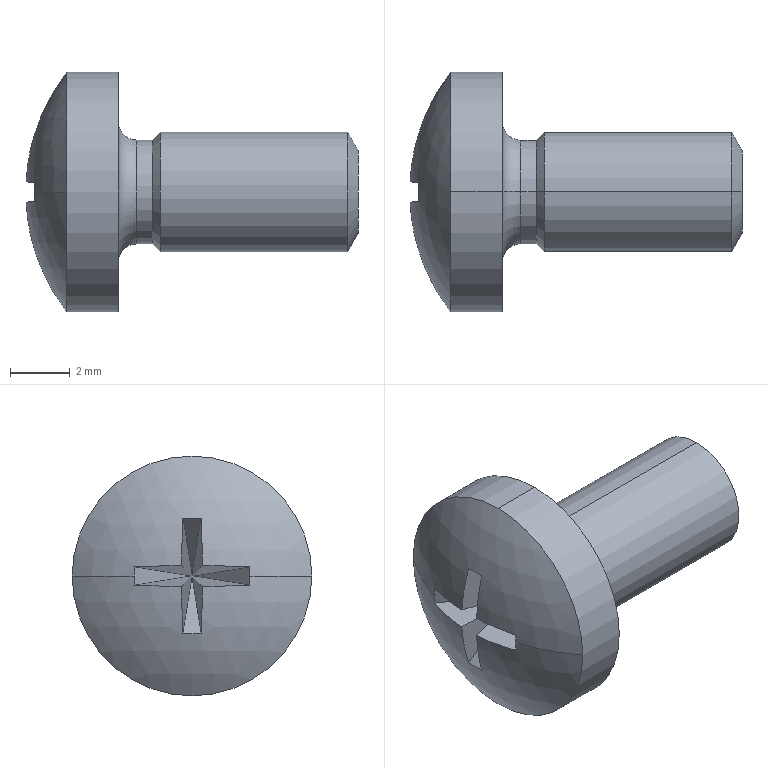Part | SolidWorks | features BlendCut 1, LPattern 1, MirrorPattern 1, RevCut 1, Revolution 1 | 1 solid | 28 faces | box 11.081 x 8 x 8 mm | volume 215 mm3 | plane 14 | cylinder 6 | cone 4 | torus 2 | sphere 2 | commonest cylinder face diameters 3.464 x2 4 x2 8 x2
STEP:
#1=CARTESIAN_POINT('',(11.1,0.,1.394));
#2=VERTEX_POINT('',#1);
#3=CARTESIAN_POINT('',(11.1,0.,-1.394));
#4=VERTEX_POINT('',#3);
#5=CARTESIAN_POINT('',(11.1,0.,0.));
#6=DIRECTION('',(-1.,0.,0.));
#7=DIRECTION('',(0.,0.,1.));
#8=AXIS2_PLACEMENT_3D('',#5,#6,#7);
#9=CIRCLE('',#8,1.394);
#10=EDGE_CURVE('',#2,#4,#9,.T.);
#11=ORIENTED_EDGE('',*,*,#10,.T.);
#12=CARTESIAN_POINT('',(10.754,0.,-2.));
#13=VERTEX_POINT('',#12);
#14=CARTESIAN_POINT('',(10.754,0.,-2.));
#15=DIRECTION('',(-0.4959,0.,-0.8684));
#16=VECTOR('',#15,1000.);
#17=LINE('',#14,#16);
#18=EDGE_CURVE('',#4,#13,#17,.T.);
#19=ORIENTED_EDGE('',*,*,#18,.T.);
#20=CARTESIAN_POINT('',(10.754,0.,2.));
#21=VERTEX_POINT('',#20);
#22=CARTESIAN_POINT('',(10.754,0.,0.));
#23=DIRECTION('',(-1.,0.,0.));
#24=DIRECTION('',(0.,0.,1.));
#25=AXIS2_PLACEMENT_3D('',#22,#23,#24);
#26=CIRCLE('',#25,2.);
#27=EDGE_CURVE('',#21,#13,#26,.T.);
#28=ORIENTED_EDGE('',*,*,#27,.F.);
#29=CARTESIAN_POINT('',(10.754,0.,2.));
#30=DIRECTION('',(-0.4959,0.,0.8684));
#31=VECTOR('',#30,1000.);
#32=LINE('',#29,#31);
#33=EDGE_CURVE('',#2,#21,#32,.T.);
#34=ORIENTED_EDGE('',*,*,#33,.F.);
#35=EDGE_LOOP('',(#11,#19,#28,#34));
#36=FACE_OUTER_BOUND('',#35,.T.);
#37=CARTESIAN_POINT('',(10.754,0.,0.));
#38=DIRECTION('',(-1.,0.,0.));
#39=DIRECTION('',(0.,0.,1.));
#40=AXIS2_PLACEMENT_3D('',#37,#38,#39);
#41=CONICAL_SURFACE('',#40,2.,1.052);
#42=ADVANCED_FACE('',(#36),#41,.T.);
#43=CARTESIAN_POINT('',(4.232,0.,1.732));
#44=VERTEX_POINT('',#43);
#45=CARTESIAN_POINT('',(4.232,0.,-1.732));
#46=VERTEX_POINT('',#45);
#47=CARTESIAN_POINT('',(4.232,0.,0.));
#48=DIRECTION('',(-1.,0.,0.));
#49=DIRECTION('',(0.,0.,1.));
#50=AXIS2_PLACEMENT_3D('',#47,#48,#49);
#51=CIRCLE('',#50,1.732);
#52=EDGE_CURVE('',#44,#46,#51,.T.);
#53=ORIENTED_EDGE('',*,*,#52,.F.);
#54=CARTESIAN_POINT('',(4.5,0.,2.));
#55=VERTEX_POINT('',#54);
#56=CARTESIAN_POINT('',(4.5,0.,2.));
#57=DIRECTION('',(0.7071,0.,0.7071));
#58=VECTOR('',#57,1000.);
#59=LINE('',#56,#58);
#60=EDGE_CURVE('',#44,#55,#59,.T.);
#61=ORIENTED_EDGE('',*,*,#60,.T.);
#62=CARTESIAN_POINT('',(4.5,0.,-2.));
#63=VERTEX_POINT('',#62);
#64=CARTESIAN_POINT('',(4.5,0.,0.));
#65=DIRECTION('',(-1.,0.,0.));
#66=DIRECTION('',(0.,0.,1.));
#67=AXIS2_PLACEMENT_3D('',#64,#65,#66);
#68=CIRCLE('',#67,2.);
#69=EDGE_CURVE('',#55,#63,#68,.T.);
#70=ORIENTED_EDGE('',*,*,#69,.T.);
#71=CARTESIAN_POINT('',(4.5,0.,-2.));
#72=DIRECTION('',(0.7071,0.,-0.7071));
#73=VECTOR('',#72,1000.);
#74=LINE('',#71,#73);
#75=EDGE_CURVE('',#46,#63,#74,.T.);
#76=ORIENTED_EDGE('',*,*,#75,.F.);
#77=EDGE_LOOP('',(#53,#61,#70,#76));
#78=FACE_OUTER_BOUND('',#77,.T.);
#79=CARTESIAN_POINT('',(4.5,0.,0.));
#80=DIRECTION('',(1.,0.,0.));
#81=DIRECTION('',(0.,0.,-1.));
#82=AXIS2_PLACEMENT_3D('',#79,#80,#81);
#83=CONICAL_SURFACE('',#82,2.,0.7854);
#84=ADVANCED_FACE('',(#78),#83,.T.);
#85=ORIENTED_EDGE('',*,*,#52,.T.);
#86=CARTESIAN_POINT('',(3.718,0.,-1.732));
#87=VERTEX_POINT('',#86);
#88=CARTESIAN_POINT('',(-1.332,0.,-1.732));
#89=DIRECTION('',(-1.,0.,0.));
#90=VECTOR('',#89,1000.);
#91=LINE('',#88,#90);
#92=EDGE_CURVE('',#46,#87,#91,.T.);
#93=ORIENTED_EDGE('',*,*,#92,.T.);
#94=CARTESIAN_POINT('',(3.718,0.,1.732));
#95=VERTEX_POINT('',#94);
#96=CARTESIAN_POINT('',(3.718,0.,0.));
#97=DIRECTION('',(-1.,0.,0.));
#98=DIRECTION('',(0.,0.,1.));
#99=AXIS2_PLACEMENT_3D('',#96,#97,#98);
#100=CIRCLE('',#99,1.732);
#101=EDGE_CURVE('',#95,#87,#100,.T.);
#102=ORIENTED_EDGE('',*,*,#101,.F.);
#103=CARTESIAN_POINT('',(-1.332,0.,1.732));
#104=DIRECTION('',(-1.,0.,0.));
#105=VECTOR('',#104,1000.);
#106=LINE('',#103,#105);
#107=EDGE_CURVE('',#44,#95,#106,.T.);
#108=ORIENTED_EDGE('',*,*,#107,.F.);
#109=EDGE_LOOP('',(#85,#93,#102,#108));
#110=FACE_OUTER_BOUND('',#109,.T.);
#111=CARTESIAN_POINT('',(-1.332,0.,0.));
#112=DIRECTION('',(-1.,0.,0.));
#113=DIRECTION('',(0.,0.,1.));
#114=AXIS2_PLACEMENT_3D('',#111,#112,#113);
#115=CYLINDRICAL_SURFACE('',#114,1.732);
#116=ADVANCED_FACE('',(#110),#115,.T.);
#117=CARTESIAN_POINT('',(3.1,0.,-2.35));
#118=VERTEX_POINT('',#117);
#119=CARTESIAN_POINT('',(3.1,0.,2.35));
#120=VERTEX_POINT('',#119);
#121=CARTESIAN_POINT('',(3.1,0.,0.));
#122=DIRECTION('',(-1.,0.,0.));
#123=DIRECTION('',(0.,0.,1.));
#124=AXIS2_PLACEMENT_3D('',#121,#122,#123);
#125=CIRCLE('',#124,2.35);
#126=EDGE_CURVE('',#118,#120,#125,.T.);
#127=ORIENTED_EDGE('',*,*,#126,.F.);
#128=CARTESIAN_POINT('',(3.718,0.,-2.35));
#129=DIRECTION('',(0.,1.,0.));
#130=DIRECTION('',(0.,0.,1.));
#131=AXIS2_PLACEMENT_3D('',#128,#129,#130);
#132=CIRCLE('',#131,0.618);
#133=EDGE_CURVE('',#118,#87,#132,.T.);
#134=ORIENTED_EDGE('',*,*,#133,.T.);
#135=CARTESIAN_POINT('',(3.718,0.,0.));
#136=DIRECTION('',(-1.,0.,0.));
#137=DIRECTION('',(0.,0.,1.));
#138=AXIS2_PLACEMENT_3D('',#135,#136,#137);
#139=CIRCLE('',#138,1.732);
#140=EDGE_CURVE('',#87,#95,#139,.T.);
#141=ORIENTED_EDGE('',*,*,#140,.T.);
#142=CARTESIAN_POINT('',(3.718,0.,2.35));
#143=DIRECTION('',(0.,-1.,0.));
#144=DIRECTION('',(0.,0.,-1.));
#145=AXIS2_PLACEMENT_3D('',#142,#143,#144);
#146=CIRCLE('',#145,0.618);
#147=EDGE_CURVE('',#120,#95,#146,.T.);
#148=ORIENTED_EDGE('',*,*,#147,.F.);
#149=EDGE_LOOP('',(#127,#134,#141,#148));
#150=FACE_OUTER_BOUND('',#149,.T.);
#151=CARTESIAN_POINT('',(3.718,0.,0.));
#152=DIRECTION('',(-1.,0.,0.));
#153=DIRECTION('',(0.,0.,1.));
#154=AXIS2_PLACEMENT_3D('',#151,#152,#153);
#155=TOROIDAL_SURFACE('',#154,2.35,0.618);
#156=ADVANCED_FACE('',(#150),#155,.F.);
#157=CARTESIAN_POINT('',(3.1,0.,4.));
#158=VERTEX_POINT('',#157);
#159=CARTESIAN_POINT('',(3.1,0.,-4.));
#160=VERTEX_POINT('',#159);
#161=CARTESIAN_POINT('',(3.1,0.,0.));
#162=DIRECTION('',(-1.,0.,0.));
#163=DIRECTION('',(0.,0.,1.));
#164=AXIS2_PLACEMENT_3D('',#161,#162,#163);
#165=CIRCLE('',#164,4.);
#166=EDGE_CURVE('',#158,#160,#165,.T.);
#167=ORIENTED_EDGE('',*,*,#166,.T.);
#168=CARTESIAN_POINT('',(1.377,0.,-4.));
#169=VERTEX_POINT('',#168);
#170=CARTESIAN_POINT('',(-1.332,0.,-4.));
#171=DIRECTION('',(-1.,0.,0.));
#172=VECTOR('',#171,1000.);
#173=LINE('',#170,#172);
#174=EDGE_CURVE('',#160,#169,#173,.T.);
#175=ORIENTED_EDGE('',*,*,#174,.T.);
#176=CARTESIAN_POINT('',(1.377,4.,0.));
#177=VERTEX_POINT('',#176);
#178=CARTESIAN_POINT('',(1.377,0.,0.));
#179=DIRECTION('',(-1.,0.,0.));
#180=DIRECTION('',(0.,0.,1.));
#181=AXIS2_PLACEMENT_3D('',#178,#179,#180);
#182=CIRCLE('',#181,4.);
#183=EDGE_CURVE('',#177,#169,#182,.T.);
#184=ORIENTED_EDGE('',*,*,#183,.F.);
#185=CARTESIAN_POINT('',(1.377,0.,4.));
#186=VERTEX_POINT('',#185);
#187=CARTESIAN_POINT('',(1.377,0.,0.));
#188=DIRECTION('',(-1.,0.,0.));
#189=DIRECTION('',(0.,0.,1.));
#190=AXIS2_PLACEMENT_3D('',#187,#188,#189);
#191=CIRCLE('',#190,4.);
#192=EDGE_CURVE('',#186,#177,#191,.T.);
#193=ORIENTED_EDGE('',*,*,#192,.F.);
#194=CARTESIAN_POINT('',(-1.332,0.,4.));
#195=DIRECTION('',(-1.,0.,0.));
#196=VECTOR('',#195,1000.);
#197=LINE('',#194,#196);
#198=EDGE_CURVE('',#158,#186,#197,.T.);
#199=ORIENTED_EDGE('',*,*,#198,.F.);
#200=EDGE_LOOP('',(#167,#175,#184,#193,#199));
#201=FACE_OUTER_BOUND('',#200,.T.);
#202=CARTESIAN_POINT('',(-1.332,0.,0.));
#203=DIRECTION('',(-1.,0.,0.));
#204=DIRECTION('',(0.,0.,1.));
#205=AXIS2_PLACEMENT_3D('',#202,#203,#204);
#206=CYLINDRICAL_SURFACE('',#205,4.);
#207=ADVANCED_FACE('',(#201),#206,.T.);
#208=ORIENTED_EDGE('',*,*,#183,.T.);
#209=CARTESIAN_POINT('',(1.377,-4.,0.));
#210=VERTEX_POINT('',#209);
#211=CARTESIAN_POINT('',(1.377,0.,0.));
#212=DIRECTION('',(-1.,0.,0.));
#213=DIRECTION('',(0.,0.,1.));
#214=AXIS2_PLACEMENT_3D('',#211,#212,#213);
#215=CIRCLE('',#214,4.);
#216=EDGE_CURVE('',#169,#210,#215,.T.);
#217=ORIENTED_EDGE('',*,*,#216,.T.);
#218=CARTESIAN_POINT('',(0.2935,-1.931,0.));
#219=VERTEX_POINT('',#218);
#220=CARTESIAN_POINT('',(6.5,0.,0.));
#221=DIRECTION('',(0.,0.,-1.));
#222=DIRECTION('',(0.,1.,0.));
#223=AXIS2_PLACEMENT_3D('',#220,#221,#222);
#224=CIRCLE('',#223,6.5);
#225=EDGE_CURVE('',#210,#219,#224,.T.);
#226=ORIENTED_EDGE('',*,*,#225,.T.);
#227=CARTESIAN_POINT('',(0.2993,-1.926,-0.3063));
#228=VERTEX_POINT('',#227);
#229=CARTESIAN_POINT('',(4.628,2.042,0.));
#230=DIRECTION('',(0.6757,-0.7372,0.));
#231=DIRECTION('',(0.7372,0.6757,0.));
#232=AXIS2_PLACEMENT_3D('',#229,#230,#231);
#233=CIRCLE('',#232,5.88);
#234=EDGE_CURVE('',#219,#228,#233,.T.);
#235=ORIENTED_EDGE('',*,*,#234,.T.);
#236=CARTESIAN_POINT('',(0.01858,-0.3473,-0.3473));
#237=VERTEX_POINT('',#236);
#238=CARTESIAN_POINT('',(6.415,0.,0.5855));
#239=DIRECTION('',(0.1443,0.,-0.9895));
#240=DIRECTION('',(-0.9895,0.,-0.1443));
#241=AXIS2_PLACEMENT_3D('',#238,#239,#240);
#242=CIRCLE('',#241,6.473);
#243=EDGE_CURVE('',#228,#237,#242,.T.);
#244=ORIENTED_EDGE('',*,*,#243,.T.);
#245=CARTESIAN_POINT('',(0.2993,-0.3063,-1.926));
#246=VERTEX_POINT('',#245);
#247=CARTESIAN_POINT('',(6.415,0.5855,0.));
#248=DIRECTION('',(0.1443,-0.9895,0.));
#249=DIRECTION('',(0.9895,0.1443,0.));
#250=AXIS2_PLACEMENT_3D('',#247,#248,#249);
#251=CIRCLE('',#250,6.473);
#252=EDGE_CURVE('',#237,#246,#251,.T.);
#253=ORIENTED_EDGE('',*,*,#252,.T.);
#254=CARTESIAN_POINT('',(0.2993,0.3063,-1.926));
#255=VERTEX_POINT('',#254);
#256=CARTESIAN_POINT('',(4.628,0.,2.042));
#257=DIRECTION('',(0.6757,0.,-0.7372));
#258=DIRECTION('',(-0.7372,0.,-0.6757));
#259=AXIS2_PLACEMENT_3D('',#256,#257,#258);
#260=CIRCLE('',#259,5.88);
#261=EDGE_CURVE('',#246,#255,#260,.T.);
#262=ORIENTED_EDGE('',*,*,#261,.T.);
#263=CARTESIAN_POINT('',(0.01858,0.3473,-0.3473));
#264=VERTEX_POINT('',#263);
#265=CARTESIAN_POINT('',(6.415,-0.5855,0.));
#266=DIRECTION('',(0.1443,0.9895,0.));
#267=DIRECTION('',(-0.9895,0.1443,0.));
#268=AXIS2_PLACEMENT_3D('',#265,#266,#267);
#269=CIRCLE('',#268,6.473);
#270=EDGE_CURVE('',#255,#264,#269,.T.);
#271=ORIENTED_EDGE('',*,*,#270,.T.);
#272=CARTESIAN_POINT('',(0.2993,1.926,-0.3063));
#273=VERTEX_POINT('',#272);
#274=CARTESIAN_POINT('',(6.415,0.,0.5855));
#275=DIRECTION('',(0.1443,0.,-0.9895));
#276=DIRECTION('',(-0.9895,0.,-0.1443));
#277=AXIS2_PLACEMENT_3D('',#274,#275,#276);
#278=CIRCLE('',#277,6.473);
#279=EDGE_CURVE('',#264,#273,#278,.T.);
#280=ORIENTED_EDGE('',*,*,#279,.T.);
#281=CARTESIAN_POINT('',(0.2935,1.931,0.));
#282=VERTEX_POINT('',#281);
#283=CARTESIAN_POINT('',(4.628,-2.042,0.));
#284=DIRECTION('',(0.6757,0.7372,0.));
#285=DIRECTION('',(-0.7372,0.6757,0.));
#286=AXIS2_PLACEMENT_3D('',#283,#284,#285);
#287=CIRCLE('',#286,5.88);
#288=EDGE_CURVE('',#273,#282,#287,.T.);
#289=ORIENTED_EDGE('',*,*,#288,.T.);
#290=CARTESIAN_POINT('',(6.5,0.,0.));
#291=DIRECTION('',(0.,0.,1.));
#292=DIRECTION('',(1.,0.,0.));
#293=AXIS2_PLACEMENT_3D('',#290,#291,#292);
#294=CIRCLE('',#293,6.5);
#295=EDGE_CURVE('',#177,#282,#294,.T.);
#296=ORIENTED_EDGE('',*,*,#295,.F.);
#297=EDGE_LOOP('',(#208,#217,#226,#235,#244,#253,#262,#271,#280,#289,#296));
#298=FACE_OUTER_BOUND('',#297,.T.);
#299=CARTESIAN_POINT('',(6.5,0.,0.));
#300=DIRECTION('',(0.,0.,-1.));
#301=DIRECTION('',(0.,1.,0.));
#302=AXIS2_PLACEMENT_3D('',#299,#300,#301);
#303=SPHERICAL_SURFACE('',#302,6.5);
#304=ADVANCED_FACE('',(#298),#303,.T.);
#305=ORIENTED_EDGE('',*,*,#27,.T.);
#306=CARTESIAN_POINT('',(-1.332,0.,-2.));
#307=DIRECTION('',(-1.,0.,0.));
#308=VECTOR('',#307,1000.);
#309=LINE('',#306,#308);
#310=EDGE_CURVE('',#13,#63,#309,.T.);
#311=ORIENTED_EDGE('',*,*,#310,.T.);
#312=ORIENTED_EDGE('',*,*,#69,.F.);
#313=CARTESIAN_POINT('',(-1.332,0.,2.));
#314=DIRECTION('',(-1.,0.,0.));
#315=VECTOR('',#314,1000.);
#316=LINE('',#313,#315);
#317=EDGE_CURVE('',#21,#55,#316,.T.);
#318=ORIENTED_EDGE('',*,*,#317,.F.);
#319=EDGE_LOOP('',(#305,#311,#312,#318));
#320=FACE_OUTER_BOUND('',#319,.T.);
#321=CARTESIAN_POINT('',(-1.332,0.,0.));
#322=DIRECTION('',(-1.,0.,0.));
#323=DIRECTION('',(0.,0.,1.));
#324=AXIS2_PLACEMENT_3D('',#321,#322,#323);
#325=CYLINDRICAL_SURFACE('',#324,2.);
#326=ADVANCED_FACE('',(#320),#325,.T.);
#327=CARTESIAN_POINT('',(2.4,0.,0.));
#328=VERTEX_POINT('',#327);
#329=CARTESIAN_POINT('',(2.4,0.,0.));
#330=DIRECTION('',(-0.7329,-0.6719,-0.1069));
#331=VECTOR('',#330,1000.);
#332=LINE('',#329,#331);
#333=EDGE_CURVE('',#328,#228,#332,.T.);
#334=ORIENTED_EDGE('',*,*,#333,.F.);
#335=CARTESIAN_POINT('',(2.4,0.,0.));
#336=DIRECTION('',(-0.9794,-0.1428,-0.1428));
#337=VECTOR('',#336,1000.);
#338=LINE('',#335,#337);
#339=EDGE_CURVE('',#328,#237,#338,.T.);
#340=ORIENTED_EDGE('',*,*,#339,.T.);
#341=ORIENTED_EDGE('',*,*,#243,.F.);
#342=EDGE_LOOP('',(#334,#340,#341));
#343=FACE_OUTER_BOUND('',#342,.T.);
#344=CARTESIAN_POINT('',(2.4,0.,0.));
#345=DIRECTION('',(0.1443,0.,-0.9895));
#346=DIRECTION('',(-0.9895,0.,-0.1443));
#347=AXIS2_PLACEMENT_3D('',#344,#345,#346);
#348=PLANE('',#347);
#349=ADVANCED_FACE('',(#343),#348,.F.);
#350=CARTESIAN_POINT('',(0.01858,-0.3473,0.3473));
#351=VERTEX_POINT('',#350);
#352=CARTESIAN_POINT('',(0.2993,-1.926,0.3063));
#353=VERTEX_POINT('',#352);
#354=CARTESIAN_POINT('',(6.415,0.,-0.5855));
#355=DIRECTION('',(0.1443,0.,0.9895));
#356=DIRECTION('',(0.9895,0.,-0.1443));
#357=AXIS2_PLACEMENT_3D('',#354,#355,#356);
#358=CIRCLE('',#357,6.473);
#359=EDGE_CURVE('',#351,#353,#358,.T.);
#360=ORIENTED_EDGE('',*,*,#359,.F.);
#361=CARTESIAN_POINT('',(2.4,0.,0.));
#362=DIRECTION('',(0.9794,0.1428,-0.1428));
#363=VECTOR('',#362,1000.);
#364=LINE('',#361,#363);
#365=EDGE_CURVE('',#351,#328,#364,.T.);
#366=ORIENTED_EDGE('',*,*,#365,.T.);
#367=CARTESIAN_POINT('',(2.4,0.,0.));
#368=DIRECTION('',(-0.7329,-0.6719,0.1069));
#369=VECTOR('',#368,1000.);
#370=LINE('',#367,#369);
#371=EDGE_CURVE('',#328,#353,#370,.T.);
#372=ORIENTED_EDGE('',*,*,#371,.T.);
#373=EDGE_LOOP('',(#360,#366,#372));
#374=FACE_OUTER_BOUND('',#373,.T.);
#375=CARTESIAN_POINT('',(2.4,0.,0.));
#376=DIRECTION('',(0.1443,0.,0.9895));
#377=DIRECTION('',(0.9895,0.,-0.1443));
#378=AXIS2_PLACEMENT_3D('',#375,#376,#377);
#379=PLANE('',#378);
#380=ADVANCED_FACE('',(#374),#379,.F.);
#381=ORIENTED_EDGE('',*,*,#310,.F.);
#382=CARTESIAN_POINT('',(10.754,0.,0.));
#383=DIRECTION('',(-1.,0.,0.));
#384=DIRECTION('',(0.,0.,1.));
#385=AXIS2_PLACEMENT_3D('',#382,#383,#384);
#386=CIRCLE('',#385,2.);
#387=EDGE_CURVE('',#13,#21,#386,.T.);
#388=ORIENTED_EDGE('',*,*,#387,.T.);
#389=ORIENTED_EDGE('',*,*,#317,.T.);
#390=CARTESIAN_POINT('',(4.5,0.,0.));
#391=DIRECTION('',(-1.,0.,0.));
#392=DIRECTION('',(0.,0.,1.));
#393=AXIS2_PLACEMENT_3D('',#390,#391,#392);
#394=CIRCLE('',#393,2.);
#395=EDGE_CURVE('',#63,#55,#394,.T.);
#396=ORIENTED_EDGE('',*,*,#395,.F.);
#397=EDGE_LOOP('',(#381,#388,#389,#396));
#398=FACE_OUTER_BOUND('',#397,.T.);
#399=CARTESIAN_POINT('',(-1.332,0.,0.));
#400=DIRECTION('',(-1.,0.,0.));
#401=DIRECTION('',(0.,0.,1.));
#402=AXIS2_PLACEMENT_3D('',#399,#400,#401);
#403=CYLINDRICAL_SURFACE('',#402,2.);
#404=ADVANCED_FACE('',(#398),#403,.T.);
#405=ORIENTED_EDGE('',*,*,#225,.F.);
#406=CARTESIAN_POINT('',(1.377,0.,0.));
#407=DIRECTION('',(-1.,0.,0.));
#408=DIRECTION('',(0.,0.,1.));
#409=AXIS2_PLACEMENT_3D('',#406,#407,#408);
#410=CIRCLE('',#409,4.);
#411=EDGE_CURVE('',#210,#186,#410,.T.);
#412=ORIENTED_EDGE('',*,*,#411,.T.);
#413=ORIENTED_EDGE('',*,*,#192,.T.);
#414=ORIENTED_EDGE('',*,*,#295,.T.);
#415=CARTESIAN_POINT('',(0.2993,1.926,0.3063));
#416=VERTEX_POINT('',#415);
#417=CARTESIAN_POINT('',(4.628,-2.042,0.));
#418=DIRECTION('',(0.6757,0.7372,0.));
#419=DIRECTION('',(-0.7372,0.6757,0.));
#420=AXIS2_PLACEMENT_3D('',#417,#418,#419);
#421=CIRCLE('',#420,5.88);
#422=EDGE_CURVE('',#282,#416,#421,.T.);
#423=ORIENTED_EDGE('',*,*,#422,.T.);
#424=CARTESIAN_POINT('',(0.01858,0.3473,0.3473));
#425=VERTEX_POINT('',#424);
#426=CARTESIAN_POINT('',(6.415,0.,-0.5855));
#427=DIRECTION('',(0.1443,0.,0.9895));
#428=DIRECTION('',(0.9895,0.,-0.1443));
#429=AXIS2_PLACEMENT_3D('',#426,#427,#428);
#430=CIRCLE('',#429,6.473);
#431=EDGE_CURVE('',#416,#425,#430,.T.);
#432=ORIENTED_EDGE('',*,*,#431,.T.);
#433=CARTESIAN_POINT('',(0.2993,0.3063,1.926));
#434=VERTEX_POINT('',#433);
#435=CARTESIAN_POINT('',(6.415,-0.5855,0.));
#436=DIRECTION('',(0.1443,0.9895,0.));
#437=DIRECTION('',(-0.9895,0.1443,0.));
#438=AXIS2_PLACEMENT_3D('',#435,#436,#437);
#439=CIRCLE('',#438,6.473);
#440=EDGE_CURVE('',#425,#434,#439,.T.);
#441=ORIENTED_EDGE('',*,*,#440,.T.);
#442=CARTESIAN_POINT('',(0.2993,-0.3063,1.926));
#443=VERTEX_POINT('',#442);
#444=CARTESIAN_POINT('',(4.628,0.,-2.042));
#445=DIRECTION('',(0.6757,0.,0.7372));
#446=DIRECTION('',(0.7372,0.,-0.6757));
#447=AXIS2_PLACEMENT_3D('',#444,#445,#446);
#448=CIRCLE('',#447,5.88);
#449=EDGE_CURVE('',#434,#443,#448,.T.);
#450=ORIENTED_EDGE('',*,*,#449,.T.);
#451=CARTESIAN_POINT('',(6.415,0.5855,0.));
#452=DIRECTION('',(0.1443,-0.9895,0.));
#453=DIRECTION('',(0.9895,0.1443,0.));
#454=AXIS2_PLACEMENT_3D('',#451,#452,#453);
#455=CIRCLE('',#454,6.473);
#456=EDGE_CURVE('',#443,#351,#455,.T.);
#457=ORIENTED_EDGE('',*,*,#456,.T.);
#458=ORIENTED_EDGE('',*,*,#359,.T.);
#459=CARTESIAN_POINT('',(4.628,2.042,0.));
#460=DIRECTION('',(0.6757,-0.7372,0.));
#461=DIRECTION('',(0.7372,0.6757,0.));
#462=AXIS2_PLACEMENT_3D('',#459,#460,#461);
#463=CIRCLE('',#462,5.88);
#464=EDGE_CURVE('',#353,#219,#463,.T.);
#465=ORIENTED_EDGE('',*,*,#464,.T.);
#466=EDGE_LOOP('',(#405,#412,#413,#414,#423,#432,#441,#450,#457,#458,#465));
#467=FACE_OUTER_BOUND('',#466,.T.);
#468=CARTESIAN_POINT('',(6.5,0.,0.));
#469=DIRECTION('',(0.,0.,-1.));
#470=DIRECTION('',(0.,1.,0.));
#471=AXIS2_PLACEMENT_3D('',#468,#469,#470);
#472=SPHERICAL_SURFACE('',#471,6.5);
#473=ADVANCED_FACE('',(#467),#472,.T.);
#474=ORIENTED_EDGE('',*,*,#174,.F.);
#475=CARTESIAN_POINT('',(3.1,0.,0.));
#476=DIRECTION('',(-1.,0.,0.));
#477=DIRECTION('',(0.,0.,1.));
#478=AXIS2_PLACEMENT_3D('',#475,#476,#477);
#479=CIRCLE('',#478,4.);
#480=EDGE_CURVE('',#160,#158,#479,.T.);
#481=ORIENTED_EDGE('',*,*,#480,.T.);
#482=ORIENTED_EDGE('',*,*,#198,.T.);
#483=ORIENTED_EDGE('',*,*,#411,.F.);
#484=ORIENTED_EDGE('',*,*,#216,.F.);
#485=EDGE_LOOP('',(#474,#481,#482,#483,#484));
#486=FACE_OUTER_BOUND('',#485,.T.);
#487=CARTESIAN_POINT('',(-1.332,0.,0.));
#488=DIRECTION('',(-1.,0.,0.));
#489=DIRECTION('',(0.,0.,1.));
#490=AXIS2_PLACEMENT_3D('',#487,#488,#489);
#491=CYLINDRICAL_SURFACE('',#490,4.);
#492=ADVANCED_FACE('',(#486),#491,.T.);
#493=ORIENTED_EDGE('',*,*,#166,.F.);
#494=ORIENTED_EDGE('',*,*,#480,.F.);
#495=EDGE_LOOP('',(#493,#494));
#496=FACE_OUTER_BOUND('',#495,.T.);
#497=CARTESIAN_POINT('',(3.1,0.,0.));
#498=DIRECTION('',(-1.,0.,0.));
#499=DIRECTION('',(0.,0.,1.));
#500=AXIS2_PLACEMENT_3D('',#497,#498,#499);
#501=CIRCLE('',#500,2.35);
#502=EDGE_CURVE('',#120,#118,#501,.T.);
#503=ORIENTED_EDGE('',*,*,#502,.T.);
#504=ORIENTED_EDGE('',*,*,#126,.T.);
#505=EDGE_LOOP('',(#503,#504));
#506=FACE_BOUND('',#505,.T.);
#507=CARTESIAN_POINT('',(3.1,2.35,0.));
#508=DIRECTION('',(-1.,0.,0.));
#509=DIRECTION('',(0.,0.,1.));
#510=AXIS2_PLACEMENT_3D('',#507,#508,#509);
#511=PLANE('',#510);
#512=ADVANCED_FACE('',(#496,#506),#511,.F.);
#513=ORIENTED_EDGE('',*,*,#133,.F.);
#514=ORIENTED_EDGE('',*,*,#502,.F.);
#515=ORIENTED_EDGE('',*,*,#147,.T.);
#516=ORIENTED_EDGE('',*,*,#101,.T.);
#517=EDGE_LOOP('',(#513,#514,#515,#516));
#518=FACE_OUTER_BOUND('',#517,.T.);
#519=CARTESIAN_POINT('',(3.718,0.,0.));
#520=DIRECTION('',(-1.,0.,0.));
#521=DIRECTION('',(0.,0.,1.));
#522=AXIS2_PLACEMENT_3D('',#519,#520,#521);
#523=TOROIDAL_SURFACE('',#522,2.35,0.618);
#524=ADVANCED_FACE('',(#518),#523,.F.);
#525=ORIENTED_EDGE('',*,*,#92,.F.);
#526=CARTESIAN_POINT('',(4.232,0.,0.));
#527=DIRECTION('',(-1.,0.,0.));
#528=DIRECTION('',(0.,0.,1.));
#529=AXIS2_PLACEMENT_3D('',#526,#527,#528);
#530=CIRCLE('',#529,1.732);
#531=EDGE_CURVE('',#46,#44,#530,.T.);
#532=ORIENTED_EDGE('',*,*,#531,.T.);
#533=ORIENTED_EDGE('',*,*,#107,.T.);
#534=ORIENTED_EDGE('',*,*,#140,.F.);
#535=EDGE_LOOP('',(#525,#532,#533,#534));
#536=FACE_OUTER_BOUND('',#535,.T.);
#537=CARTESIAN_POINT('',(-1.332,0.,0.));
#538=DIRECTION('',(-1.,0.,0.));
#539=DIRECTION('',(0.,0.,1.));
#540=AXIS2_PLACEMENT_3D('',#537,#538,#539);
#541=CYLINDRICAL_SURFACE('',#540,1.732);
#542=ADVANCED_FACE('',(#536),#541,.T.);
#543=ORIENTED_EDGE('',*,*,#60,.F.);
#544=ORIENTED_EDGE('',*,*,#531,.F.);
#545=ORIENTED_EDGE('',*,*,#75,.T.);
#546=ORIENTED_EDGE('',*,*,#395,.T.);
#547=EDGE_LOOP('',(#543,#544,#545,#546));
#548=FACE_OUTER_BOUND('',#547,.T.);
#549=CARTESIAN_POINT('',(4.5,0.,0.));
#550=DIRECTION('',(1.,0.,0.));
#551=DIRECTION('',(0.,0.,-1.));
#552=AXIS2_PLACEMENT_3D('',#549,#550,#551);
#553=CONICAL_SURFACE('',#552,2.,0.7854);
#554=ADVANCED_FACE('',(#548),#553,.T.);
#555=ORIENTED_EDGE('',*,*,#18,.F.);
#556=CARTESIAN_POINT('',(11.1,0.,0.));
#557=DIRECTION('',(-1.,0.,0.));
#558=DIRECTION('',(0.,0.,1.));
#559=AXIS2_PLACEMENT_3D('',#556,#557,#558);
#560=CIRCLE('',#559,1.394);
#561=EDGE_CURVE('',#4,#2,#560,.T.);
#562=ORIENTED_EDGE('',*,*,#561,.T.);
#563=ORIENTED_EDGE('',*,*,#33,.T.);
#564=ORIENTED_EDGE('',*,*,#387,.F.);
#565=EDGE_LOOP('',(#555,#562,#563,#564));
#566=FACE_OUTER_BOUND('',#565,.T.);
#567=CARTESIAN_POINT('',(10.754,0.,0.));
#568=DIRECTION('',(-1.,0.,0.));
#569=DIRECTION('',(0.,0.,1.));
#570=AXIS2_PLACEMENT_3D('',#567,#568,#569);
#571=CONICAL_SURFACE('',#570,2.,1.052);
#572=ADVANCED_FACE('',(#566),#571,.T.);
#573=ORIENTED_EDGE('',*,*,#10,.F.);
#574=ORIENTED_EDGE('',*,*,#561,.F.);
#575=EDGE_LOOP('',(#573,#574));
#576=FACE_OUTER_BOUND('',#575,.T.);
#577=CARTESIAN_POINT('',(11.1,0.,0.));
#578=DIRECTION('',(-1.,0.,0.));
#579=DIRECTION('',(0.,0.,1.));
#580=AXIS2_PLACEMENT_3D('',#577,#578,#579);
#581=PLANE('',#580);
#582=ADVANCED_FACE('',(#576),#581,.F.);
#583=ORIENTED_EDGE('',*,*,#279,.F.);
#584=CARTESIAN_POINT('',(2.4,0.,0.));
#585=DIRECTION('',(0.9794,-0.1428,0.1428));
#586=VECTOR('',#585,1000.);
#587=LINE('',#584,#586);
#588=EDGE_CURVE('',#264,#328,#587,.T.);
#589=ORIENTED_EDGE('',*,*,#588,.T.);
#590=CARTESIAN_POINT('',(2.4,0.,0.));
#591=DIRECTION('',(-0.7329,0.6719,-0.1069));
#592=VECTOR('',#591,1000.);
#593=LINE('',#590,#592);
#594=EDGE_CURVE('',#328,#273,#593,.T.);
#595=ORIENTED_EDGE('',*,*,#594,.T.);
#596=EDGE_LOOP('',(#583,#589,#595));
#597=FACE_OUTER_BOUND('',#596,.T.);
#598=CARTESIAN_POINT('',(2.4,0.,0.));
#599=DIRECTION('',(0.1443,0.,-0.9895));
#600=DIRECTION('',(-0.9895,0.,-0.1443));
#601=AXIS2_PLACEMENT_3D('',#598,#599,#600);
#602=PLANE('',#601);
#603=ADVANCED_FACE('',(#597),#602,.F.);
#604=ORIENTED_EDGE('',*,*,#594,.F.);
#605=CARTESIAN_POINT('',(2.4,0.,0.));
#606=DIRECTION('',(-0.7329,0.6719,0.1069));
#607=VECTOR('',#606,1000.);
#608=LINE('',#605,#607);
#609=EDGE_CURVE('',#328,#416,#608,.T.);
#610=ORIENTED_EDGE('',*,*,#609,.T.);
#611=ORIENTED_EDGE('',*,*,#422,.F.);
#612=ORIENTED_EDGE('',*,*,#288,.F.);
#613=EDGE_LOOP('',(#604,#610,#611,#612));
#614=FACE_OUTER_BOUND('',#613,.T.);
#615=CARTESIAN_POINT('',(0.,2.2,-0.35));
#616=DIRECTION('',(0.6757,0.7372,0.));
#617=DIRECTION('',(-0.7372,0.6757,0.));
#618=AXIS2_PLACEMENT_3D('',#615,#616,#617);
#619=PLANE('',#618);
#620=ADVANCED_FACE('',(#614),#619,.F.);
#621=ORIENTED_EDGE('',*,*,#371,.F.);
#622=ORIENTED_EDGE('',*,*,#333,.T.);
#623=ORIENTED_EDGE('',*,*,#234,.F.);
#624=ORIENTED_EDGE('',*,*,#464,.F.);
#625=EDGE_LOOP('',(#621,#622,#623,#624));
#626=FACE_OUTER_BOUND('',#625,.T.);
#627=CARTESIAN_POINT('',(0.,-2.2,0.35));
#628=DIRECTION('',(0.6757,-0.7372,0.));
#629=DIRECTION('',(0.7372,0.6757,0.));
#630=AXIS2_PLACEMENT_3D('',#627,#628,#629);
#631=PLANE('',#630);
#632=ADVANCED_FACE('',(#626),#631,.F.);
#633=ORIENTED_EDGE('',*,*,#609,.F.);
#634=CARTESIAN_POINT('',(2.4,0.,0.));
#635=DIRECTION('',(-0.9794,0.1428,0.1428));
#636=VECTOR('',#635,1000.);
#637=LINE('',#634,#636);
#638=EDGE_CURVE('',#328,#425,#637,.T.);
#639=ORIENTED_EDGE('',*,*,#638,.T.);
#640=ORIENTED_EDGE('',*,*,#431,.F.);
#641=EDGE_LOOP('',(#633,#639,#640));
#642=FACE_OUTER_BOUND('',#641,.T.);
#643=CARTESIAN_POINT('',(2.4,0.,0.));
#644=DIRECTION('',(0.1443,0.,0.9895));
#645=DIRECTION('',(0.9895,0.,-0.1443));
#646=AXIS2_PLACEMENT_3D('',#643,#644,#645);
#647=PLANE('',#646);
#648=ADVANCED_FACE('',(#642),#647,.F.);
#649=CARTESIAN_POINT('',(2.4,0.,0.));
#650=DIRECTION('',(-0.7329,-0.1069,0.6719));
#651=VECTOR('',#650,1000.);
#652=LINE('',#649,#651);
#653=EDGE_CURVE('',#328,#443,#652,.T.);
#654=ORIENTED_EDGE('',*,*,#653,.F.);
#655=ORIENTED_EDGE('',*,*,#365,.F.);
#656=ORIENTED_EDGE('',*,*,#456,.F.);
#657=EDGE_LOOP('',(#654,#655,#656));
#658=FACE_OUTER_BOUND('',#657,.T.);
#659=CARTESIAN_POINT('',(2.4,0.,0.));
#660=DIRECTION('',(0.1443,-0.9895,0.));
#661=DIRECTION('',(-0.9895,-0.1443,0.));
#662=AXIS2_PLACEMENT_3D('',#659,#660,#661);
#663=PLANE('',#662);
#664=ADVANCED_FACE('',(#658),#663,.F.);
#665=ORIENTED_EDGE('',*,*,#638,.F.);
#666=CARTESIAN_POINT('',(2.4,0.,0.));
#667=DIRECTION('',(-0.7329,0.1069,0.6719));
#668=VECTOR('',#667,1000.);
#669=LINE('',#666,#668);
#670=EDGE_CURVE('',#328,#434,#669,.T.);
#671=ORIENTED_EDGE('',*,*,#670,.T.);
#672=ORIENTED_EDGE('',*,*,#440,.F.);
#673=EDGE_LOOP('',(#665,#671,#672));
#674=FACE_OUTER_BOUND('',#673,.T.);
#675=CARTESIAN_POINT('',(2.4,0.,0.));
#676=DIRECTION('',(0.1443,0.9895,0.));
#677=DIRECTION('',(0.9895,-0.1443,0.));
#678=AXIS2_PLACEMENT_3D('',#675,#676,#677);
#679=PLANE('',#678);
#680=ADVANCED_FACE('',(#674),#679,.F.);
#681=ORIENTED_EDGE('',*,*,#670,.F.);
#682=ORIENTED_EDGE('',*,*,#653,.T.);
#683=ORIENTED_EDGE('',*,*,#449,.F.);
#684=EDGE_LOOP('',(#681,#682,#683));
#685=FACE_OUTER_BOUND('',#684,.T.);
#686=CARTESIAN_POINT('',(0.,-0.35,2.2));
#687=DIRECTION('',(0.6757,0.,0.7372));
#688=DIRECTION('',(-0.7372,0.,0.6757));
#689=AXIS2_PLACEMENT_3D('',#686,#687,#688);
#690=PLANE('',#689);
#691=ADVANCED_FACE('',(#685),#690,.F.);
#692=ORIENTED_EDGE('',*,*,#339,.F.);
#693=CARTESIAN_POINT('',(2.4,0.,0.));
#694=DIRECTION('',(-0.7329,-0.1069,-0.6719));
#695=VECTOR('',#694,1000.);
#696=LINE('',#693,#695);
#697=EDGE_CURVE('',#328,#246,#696,.T.);
#698=ORIENTED_EDGE('',*,*,#697,.T.);
#699=ORIENTED_EDGE('',*,*,#252,.F.);
#700=EDGE_LOOP('',(#692,#698,#699));
#701=FACE_OUTER_BOUND('',#700,.T.);
#702=CARTESIAN_POINT('',(2.4,0.,0.));
#703=DIRECTION('',(0.1443,-0.9895,0.));
#704=DIRECTION('',(-0.9895,-0.1443,0.));
#705=AXIS2_PLACEMENT_3D('',#702,#703,#704);
#706=PLANE('',#705);
#707=ADVANCED_FACE('',(#701),#706,.F.);
#708=ORIENTED_EDGE('',*,*,#697,.F.);
#709=CARTESIAN_POINT('',(2.4,0.,0.));
#710=DIRECTION('',(-0.7329,0.1069,-0.6719));
#711=VECTOR('',#710,1000.);
#712=LINE('',#709,#711);
#713=EDGE_CURVE('',#328,#255,#712,.T.);
#714=ORIENTED_EDGE('',*,*,#713,.T.);
#715=ORIENTED_EDGE('',*,*,#261,.F.);
#716=EDGE_LOOP('',(#708,#714,#715));
#717=FACE_OUTER_BOUND('',#716,.T.);
#718=CARTESIAN_POINT('',(0.,0.35,-2.2));
#719=DIRECTION('',(0.6757,0.,-0.7372));
#720=DIRECTION('',(0.7372,0.,0.6757));
#721=AXIS2_PLACEMENT_3D('',#718,#719,#720);
#722=PLANE('',#721);
#723=ADVANCED_FACE('',(#717),#722,.F.);
#724=ORIENTED_EDGE('',*,*,#713,.F.);
#725=ORIENTED_EDGE('',*,*,#588,.F.);
#726=ORIENTED_EDGE('',*,*,#270,.F.);
#727=EDGE_LOOP('',(#724,#725,#726));
#728=FACE_OUTER_BOUND('',#727,.T.);
#729=CARTESIAN_POINT('',(2.4,0.,0.));
#730=DIRECTION('',(0.1443,0.9895,0.));
#731=DIRECTION('',(0.9895,-0.1443,0.));
#732=AXIS2_PLACEMENT_3D('',#729,#730,#731);
#733=PLANE('',#732);
#734=ADVANCED_FACE('',(#728),#733,.F.);
#735=CLOSED_SHELL('',(#42,#84,#116,#156,#207,#304,#326,#349,#380,#404,#473,#492,#512,#524,#542,#554,#572,#582,#603,#620,#632,#648,#664,#680,#691,#707,#723,#734));
#736=MANIFOLD_SOLID_BREP('',#735);
#737=CARTESIAN_POINT('',(0.,0.,0.));
#738=DIRECTION('',(0.,0.,1.));
#739=DIRECTION('',(1.,0.,0.));
#740=AXIS2_PLACEMENT_3D('',#737,#738,#739);
#741=(LENGTH_UNIT()NAMED_UNIT(*)SI_UNIT(.MILLI.,.METRE.));
#742=UNCERTAINTY_MEASURE_WITH_UNIT(LENGTH_MEASURE(0.00001),#741,'','');
#743=(NAMED_UNIT(*)PLANE_ANGLE_UNIT()SI_UNIT($,.RADIAN.));
#744=(NAMED_UNIT(*)SI_UNIT($,.STERADIAN.)SOLID_ANGLE_UNIT());
#745=(GEOMETRIC_REPRESENTATION_CONTEXT(3)GLOBAL_UNCERTAINTY_ASSIGNED_CONTEXT((#742))GLOBAL_UNIT_ASSIGNED_CONTEXT((#741,#743,#744))REPRESENTATION_CONTEXT('',''));
#746=ADVANCED_BREP_SHAPE_REPRESENTATION('',(#736,#740),#745);